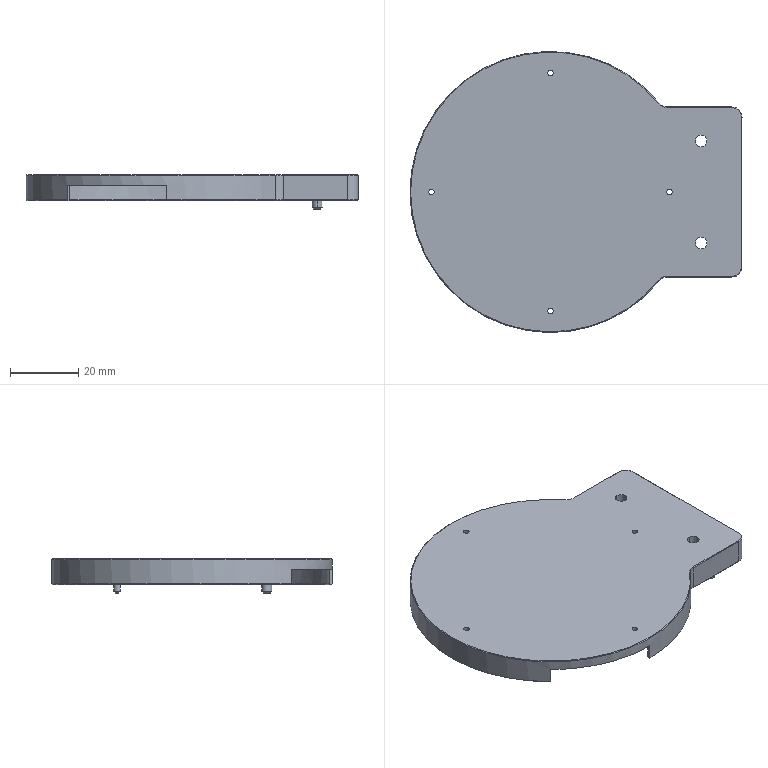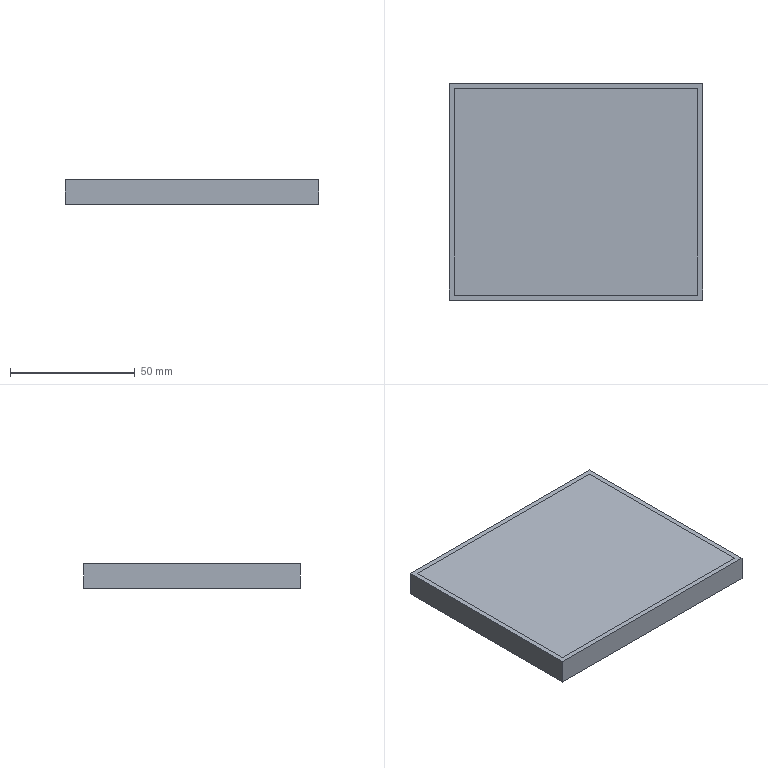CAM job | NX | 3-axis milling, drilling | part box 97.6 x 82.6 x 10 mm | stock box 101.6 x 86.6 x 10 mm
Tools:
number,name,description,diameter,corner_radius,flute_length,length,flutes
1,D6A45,Milling Tool-5 Parameters,6.0,0.0,50.0,75.0,2
16,1.6ZT,Drilling Tool,1.6,0.0,35.0,50.0,2
3,3.4ZT,Drilling Tool,3.4,0.0,35.0,50.0,2
15,D10,Milling Tool-5 Parameters,10.0,0.0,50.0,75.0,2
12,D6,Milling Tool-5 Parameters,6.0,0.0,50.0,75.0,2
14,D10JING,Milling Tool-5 Parameters,10.0,0.0,50.0,75.0,2
17,D3,Milling Tool-5 Parameters,3.0,0.0,50.0,75.0,2
Operations:
program,operation,operation_type,tool,method,geometry_group,spindle_rpm,surface_speed,feed_per_tooth,feed_cut,feed_plunge,cut_length_mm,path_length_mm,cut_time_min,machine_time_min
1,DRILLING_COPY_1,Operation,D6A45,METHOD,A,5000.0,94.0,0.035,350.0,0.0,24.6,306.989,0.0703,0.0985
1,DRILLING_COPY_1_COPY_COPY,Operation,1.6ZT,METHOD,A,2000.0,12.0,0.0375,150.0,0.0,31.923,281.61,0.2128,0.2378
1,DRILLING_COPY_1_COPY_1_1_COPY_1,Operation,3.4ZT,METHOD,A,2000.0,34.0,0.05,200.0,0.0,26.043,145.236,0.1302,0.1421
1,ZLEVEL_PROFILE,ZLevelMilling,D10,METHOD,A,9500.0,298.0,0.1684,3200.0,1000.0,3416.582,3482.982,1.1,1.106
1,ZLEVEL_PROFILE_2,ZLevelMilling,D6,METHOD,A,9500.0,179.0,0.0842,1600.0,100.0,145.558,407.256,0.091,0.1171
1,PLANAR_MILL_COPY_COPY_COPY_COPY_COPY_COPY_1_COPY_1,PlanarMilling,D6A45,METHOD,A,9500.0,179.0,0.0658,1250.0,100.0,329.192,557.013,0.2634,0.2861
1,ZLEVEL_PROFILE_COPY_1_COPY_COPY_1_COPY_COPY,ZLevelMilling,D10JING,METHOD,A,9500.0,298.0,0.0632,1200.0,1000.0,1333.776,1411.201,1.112,1.119
2,CAVITY_MILL,CavityMilling,D10,METHOD,B,9500.0,298.0,0.1316,2500.0,1000.0,10896.032,11688.353,4.86,4.939
2,CAVITY_MILL_COPY,CavityMilling,D6,METHOD,B,9500.0,179.0,0.0789,1500.0,1000.0,2213.311,3823.222,1.835,1.996
2,FLOOR_WALL,VolumeBased25DMillingOperation,D6,METHOD,B,9500.0,179.0,0.0579,1100.0,100.0,3677.197,5270.617,3.343,3.502
2,CAVITY_MILL_COPY_COPY,CavityMilling,D3,METHOD,B,9500.0,89.0,0.0579,1100.0,1000.0,2280.038,4298.906,2.171,2.373
2,PLANAR_MILL_COPY_COPY_COPY_COPY_COPY_COPY_1_COPY_1_1,PlanarMilling,D6A45,METHOD,B,9500.0,179.0,0.0658,1250.0,100.0,702.19,1410.825,0.5618,0.6326
2,DRILLING_COPY_1_COPY,Operation,D6A45,METHOD,B,5000.0,94.0,0.035,350.0,0.0,17.2,266.165,0.0491,0.074
2,PLANAR_MILL_COPY_COPY_COPY_COPY_COPY_COPY_1_COPY_1_1_COPY,PlanarMilling,D6A45,METHOD,B,9500.0,179.0,0.0658,1250.0,100.0,66.442,228.024,0.0532,0.0693